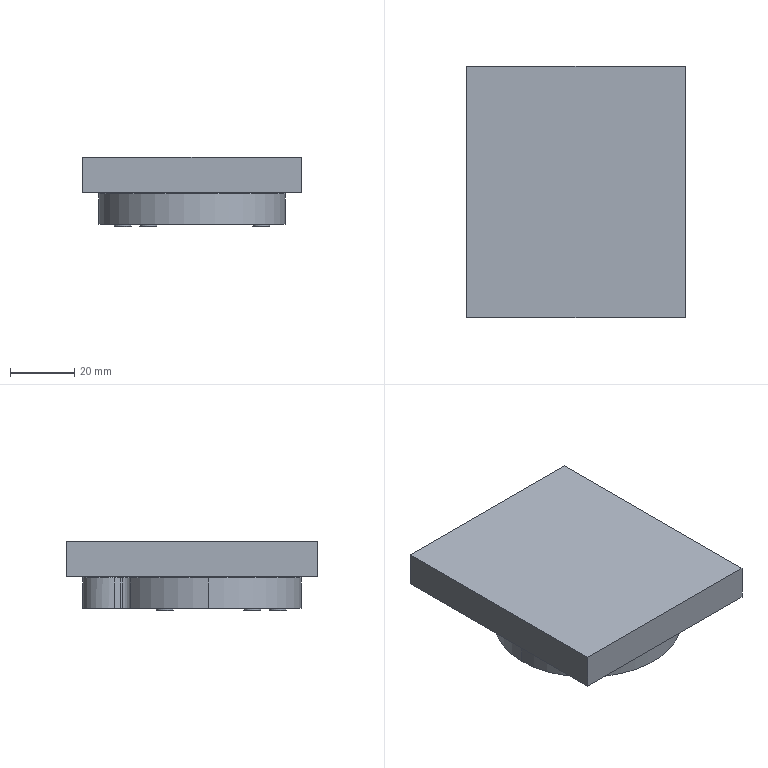Part | 2 solids | 155 faces | box 68 x 78.27 x 21.8 mm | volume 51052 mm3 | cylinder 81 | plane 41 | cone 26 | torus 7 | commonest cylinder face diameters 4 x18 6 x11 3.5 x6 5.3 x6 2 x5 54 x5